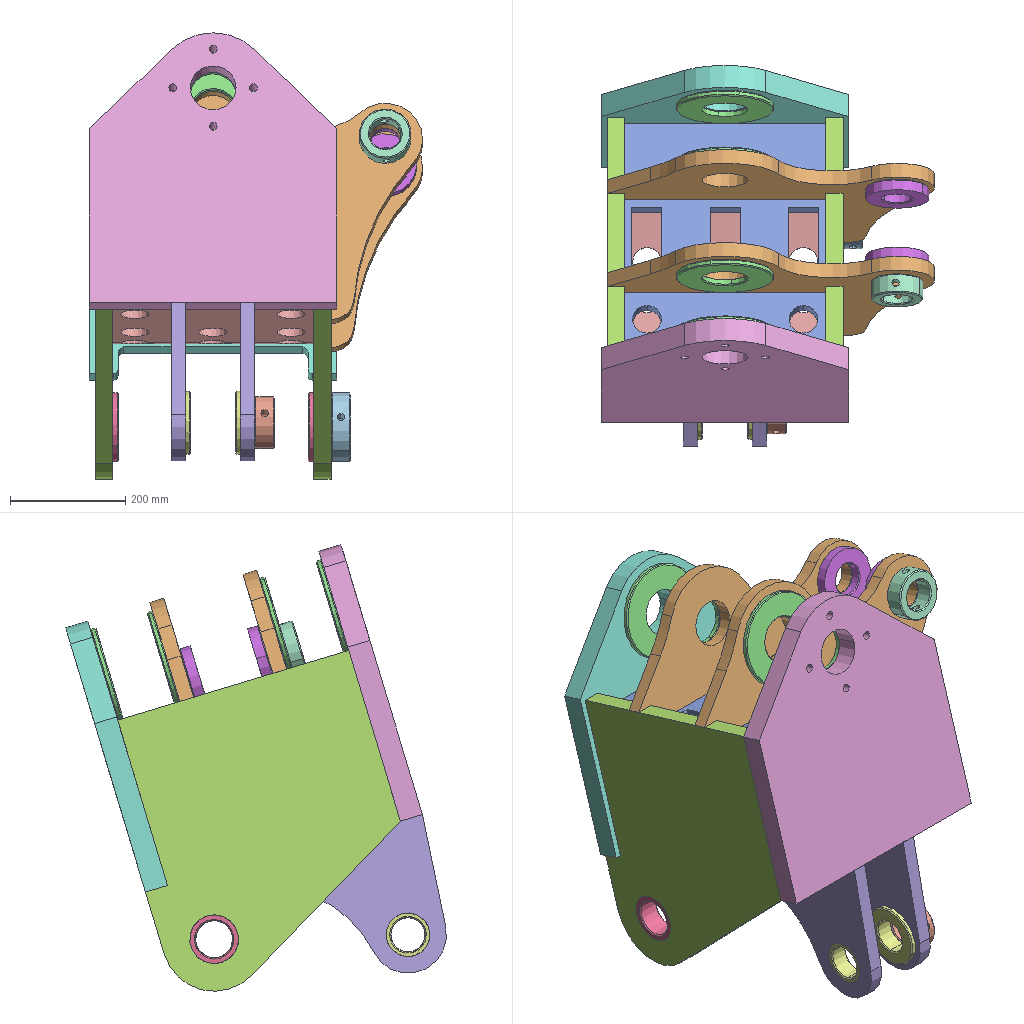Assembly | SolidWorks | 14 different items | 23 placed | box 579 x 662 x 777 mm
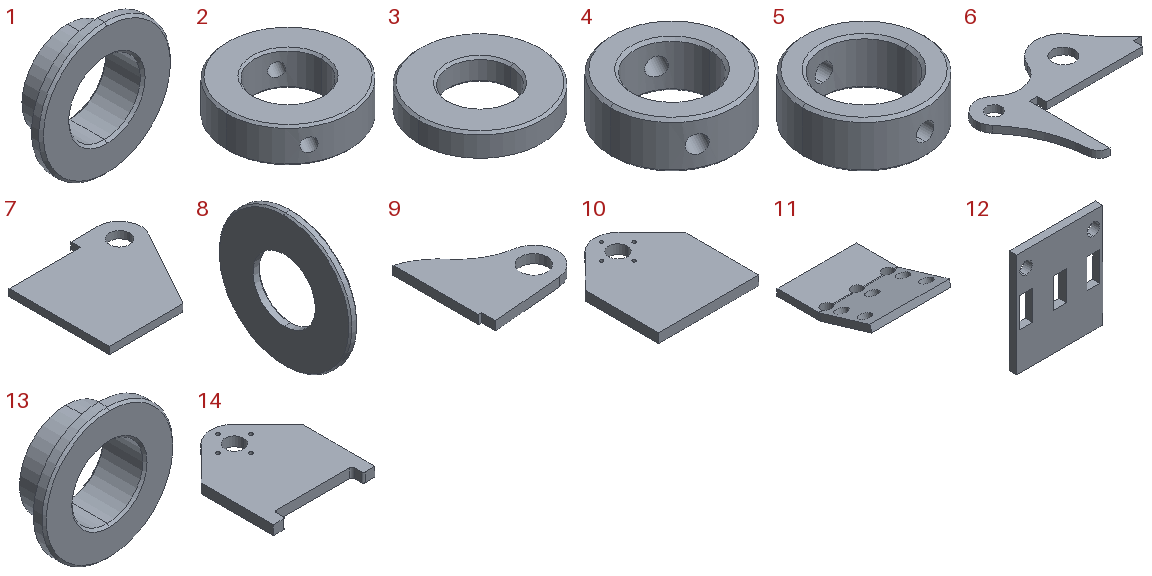Parts list (item | quantity | size | volume | features):
1 | x2 | 110 x 33 x 110 mm | 94679 mm3 | features Chamfer 1, Revolution 1
2 | x1 | 120 x 120 x 34 mm | 262064 mm3 | features 3DProfileFeature 1, Chamfer 1, Extrusion 1, HoleWzd 1
3 | x2 | 110 x 110 x 20 mm | 141159 mm3 | features Chamfer 1, Extrusion 1
4 | x1 | 90 x 90 x 34 mm | 127902 mm3 | features 3DProfileFeature 1, Chamfer 1, Extrusion 1, HoleWzd 1
5 | x1 | 90 x 90 x 34 mm | 114282 mm3 | features Chamfer 1, Extrusion 1, ICE 1
6 | x2 | 569.4 x 475 x 25 mm | 2079428 mm3 | features Extrusion 1
7 | x2 | 503.5 x 460 x 30 mm | 5359945 mm3 | features Extrusion 1
8 | x4 | 10 x 170 x 170 mm | 174084 mm3 | features Chamfer 1, Extrusion 1
9 | x2 | 270 x 282.5 x 25 mm | 1101150 mm3 | features Extrusion 1
10 | x1 | 430.2 x 490 x 40 mm | 6980590 mm3 | features Extrusion 1, HoleWzd 1
11 | x1 | 350 x 419.833 x 98.276 mm | 3997529 mm3 | features FlatPattern 1, SM3dBend 1, SMBaseFlange 1, SheetMetal 1
12 | x1 | 350 x 30 x 420 mm | 3719790 mm3 | features Extrusion 1
13 | x2 | 120 x 40 x 120 mm | 149021 mm3 | features Chamfer 1, Revolution 1
14 | x1 | 430.2 x 480 x 40 mm | 6175144 mm3 | features Extrusion 1, HoleWzd 1
Mates (type | each side: item.copy, entity, surface, feature):
DistanceDim | 12.1 face plane Boss-Extrude1 | 11.1 face plane Sketched Bend1
Coincident | 11.1 face plane Base-Flange1 | 12.1 face plane Boss-Extrude1 | 2 times
DistanceDim | 7.1 face plane Boss-Extrude1 | 11.1 face plane Base-Flange1
DistanceDim | 7.1 face plane Boss-Extrude1 | 12.1 face plane Boss-Extrude1
Coincident | 12.1 face plane Boss-Extrude1 | 7.1 face plane Boss-Extrude1
Coincident | 7.1 face plane Boss-Extrude1 | 10.1 face plane Boss-Extrude1
DistanceDim | 10.1 face plane Boss-Extrude1 | 7.1 face plane Boss-Extrude1
Coincident | 7.1 vertex | 10.1 face plane Boss-Extrude1
Coincident | 12.1 face plane Boss-Extrude1 | 14.1 face plane Boss-Extrude1
Coincident | 7.1 face plane Boss-Extrude1 | 14.1 face plane Boss-Extrude1
Coincident | 10.1 face plane Boss-Extrude1 | 14.1 face plane Boss-Extrude1
DistanceDim | 14.1 face plane Boss-Extrude1 | 6.1 face plane Boss-Extrude1
Coincident | 7.1 face plane Boss-Extrude1 | 6.1 face plane Boss-Extrude1 | 2 times
DistanceDim | 6.2 face plane Boss-Extrude1 | 10.1 face plane Boss-Extrude1
Coincident | 7.1 face plane Boss-Extrude1 | 6.2 face plane Boss-Extrude1 | 2 times
DistanceDim | 9.1 face plane Boss-Extrude1 | 10.1 face plane Boss-Extrude1
Coincident | 10.1 face plane Boss-Extrude1 | 9.1 face plane Boss-Extrude1
Coincident | 11.1 face plane Sketched Bend1 | 9.1 face plane Boss-Extrude1
DistanceDim | 9.2 face plane Boss-Extrude1 | 10.1 face plane Boss-Extrude1
Coincident | 11.1 face plane Sketched Bend1 | 9.2 face plane Boss-Extrude1
Coincident | 10.1 face plane Boss-Extrude1 | 9.2 face plane Boss-Extrude1
Concentric | 14.1 face cylinder Boss-Extrude1 | 8.1 face cylinder Boss-Extrude1
Coincident | 14.1 face plane Boss-Extrude1 | 8.1 face plane Boss-Extrude1
Coincident | 6.1 face plane Boss-Extrude1 | 8.2 face plane Boss-Extrude1
Coincident | 6.1 face cylinder Boss-Extrude1 | 8.2 edge
Concentric | 6.2 face cylinder Boss-Extrude1 | 8.3 face cylinder Boss-Extrude1
Coincident | 6.2 face plane Boss-Extrude1 | 8.3 face plane Boss-Extrude1
Concentric | 10.1 face cylinder Boss-Extrude1 | 8.4 face cylinder Boss-Extrude1
Coincident | 10.1 face plane Boss-Extrude1 | 8.4 face plane Boss-Extrude1
Concentric | 7.2 face cylinder Boss-Extrude1 | 13.1 face cylinder Revolve1
Coincident | 7.2 face plane Boss-Extrude1 | 13.1 face plane Revolve1
Concentric | 7.1 face cylinder Boss-Extrude1 | 13.2 face cylinder Revolve1
Coincident | 7.1 face plane Boss-Extrude1 | 13.2 face plane Revolve1
Concentric | 13.2 face cylinder Revolve1 | 2.1 face cylinder Boss-Extrude1
Coincident | 7.1 face plane Boss-Extrude1 | 2.1 face plane Boss-Extrude1
Concentric | 9.2 face cylinder Boss-Extrude1 | 1.1 face cylinder Revolve1
Coincident | 9.2 face plane Boss-Extrude1 | 1.1 face plane Revolve1
Concentric | 9.1 face cylinder Boss-Extrude1 | 1.2 face cylinder Revolve1
Coincident | 9.1 face plane Boss-Extrude1 | 1.2 face plane Revolve1
Concentric | 6.1 face cylinder Boss-Extrude1 | 3.1 face cylinder Boss-Extrude1
Coincident | 6.1 face plane Boss-Extrude1 | 3.1 face plane Boss-Extrude1
Concentric | 6.2 face cylinder Boss-Extrude1 | 3.2 face cylinder Boss-Extrude1
Coincident | 6.2 face plane Boss-Extrude1 | 3.2 face plane Boss-Extrude1
Concentric | 6.2 face cylinder Boss-Extrude1 | 4.1 face cylinder Boss-Extrude1
Coincident | 6.2 face plane Boss-Extrude1 | 4.1 face plane Boss-Extrude1
Concentric | 1.2 face cylinder Revolve1 | 5.1 face cylinder Boss-Extrude1
Coincident | 9.1 face plane Boss-Extrude1 | 5.1 face plane Boss-Extrude1